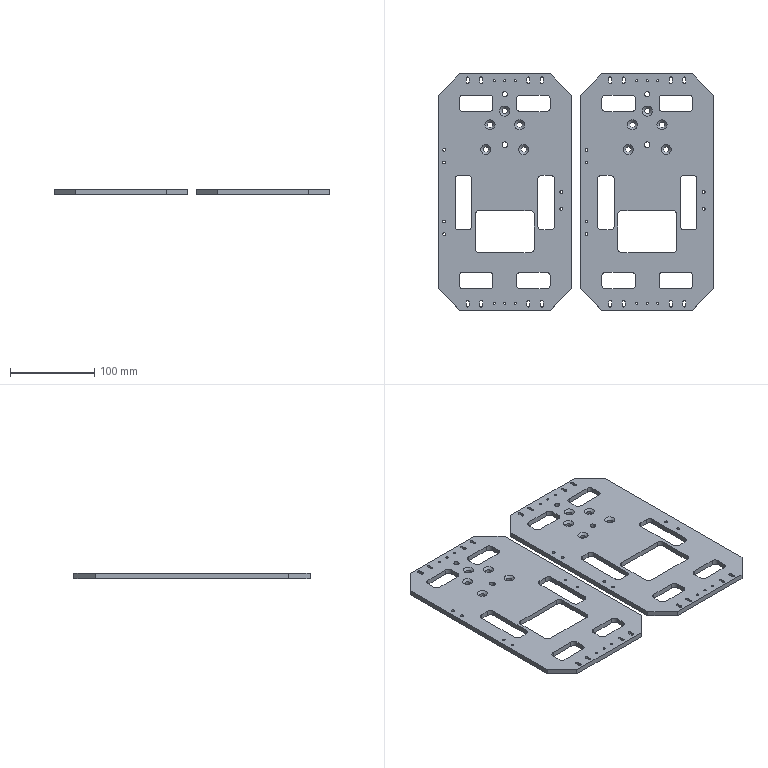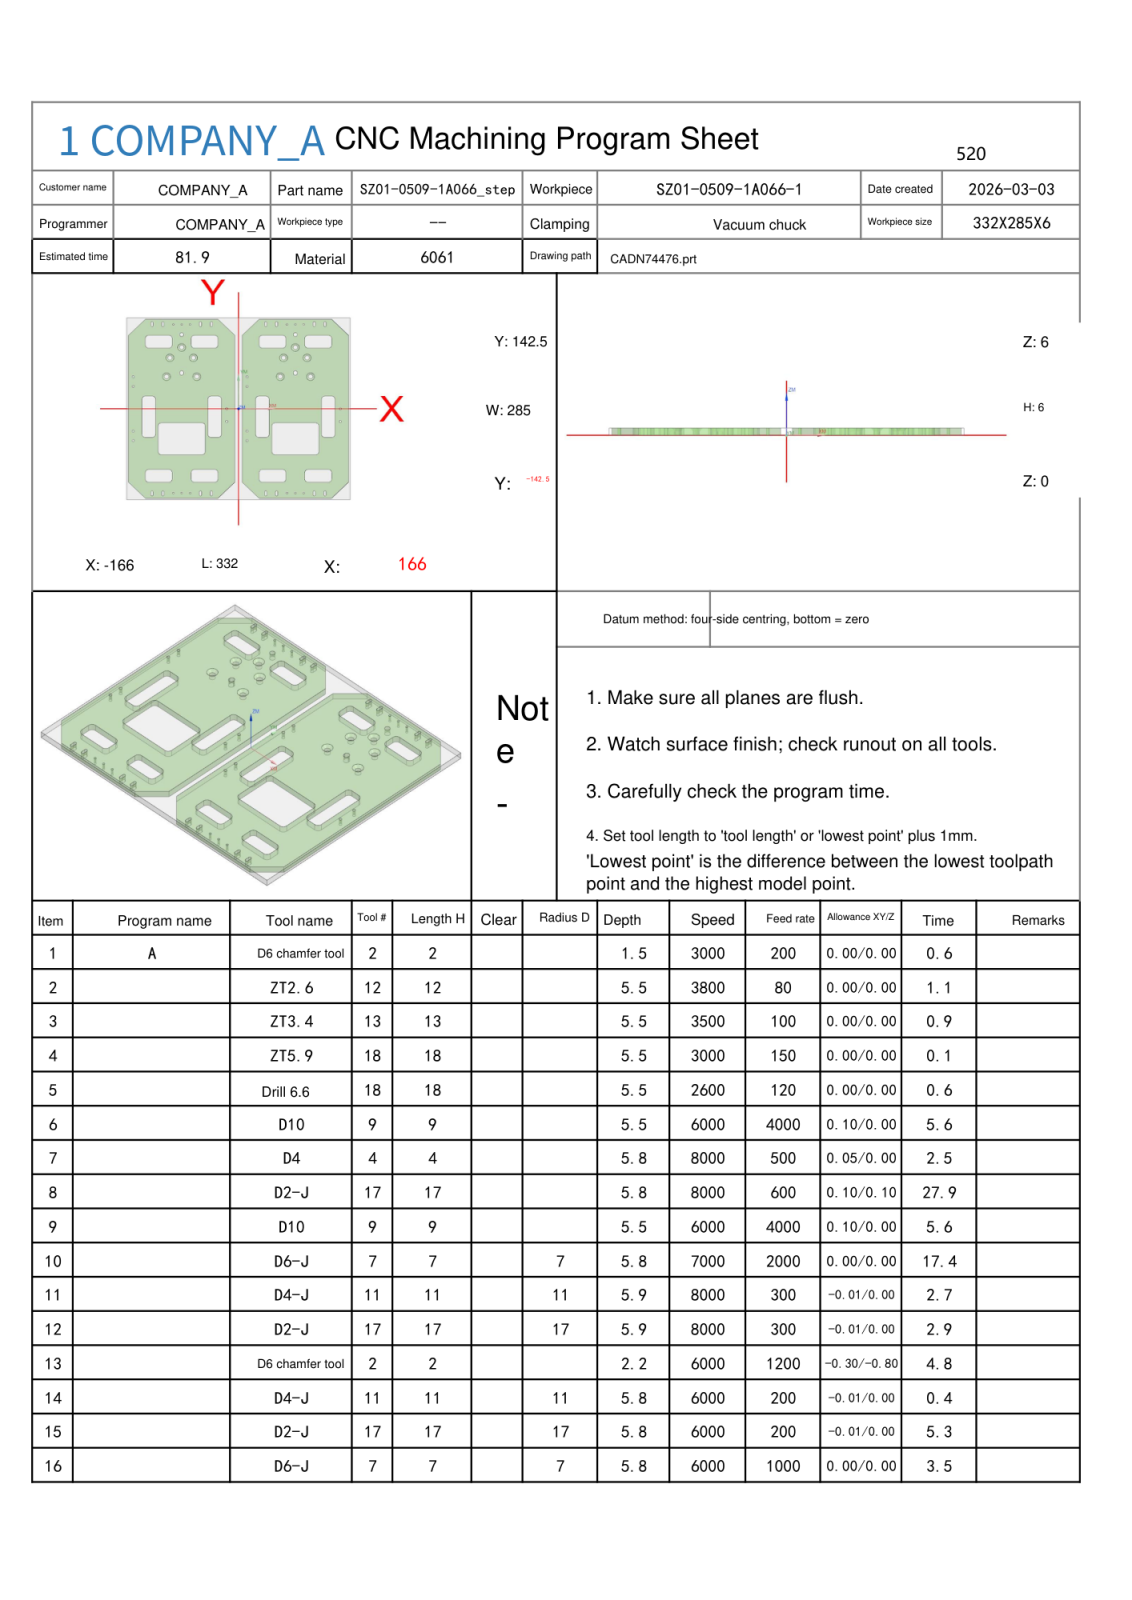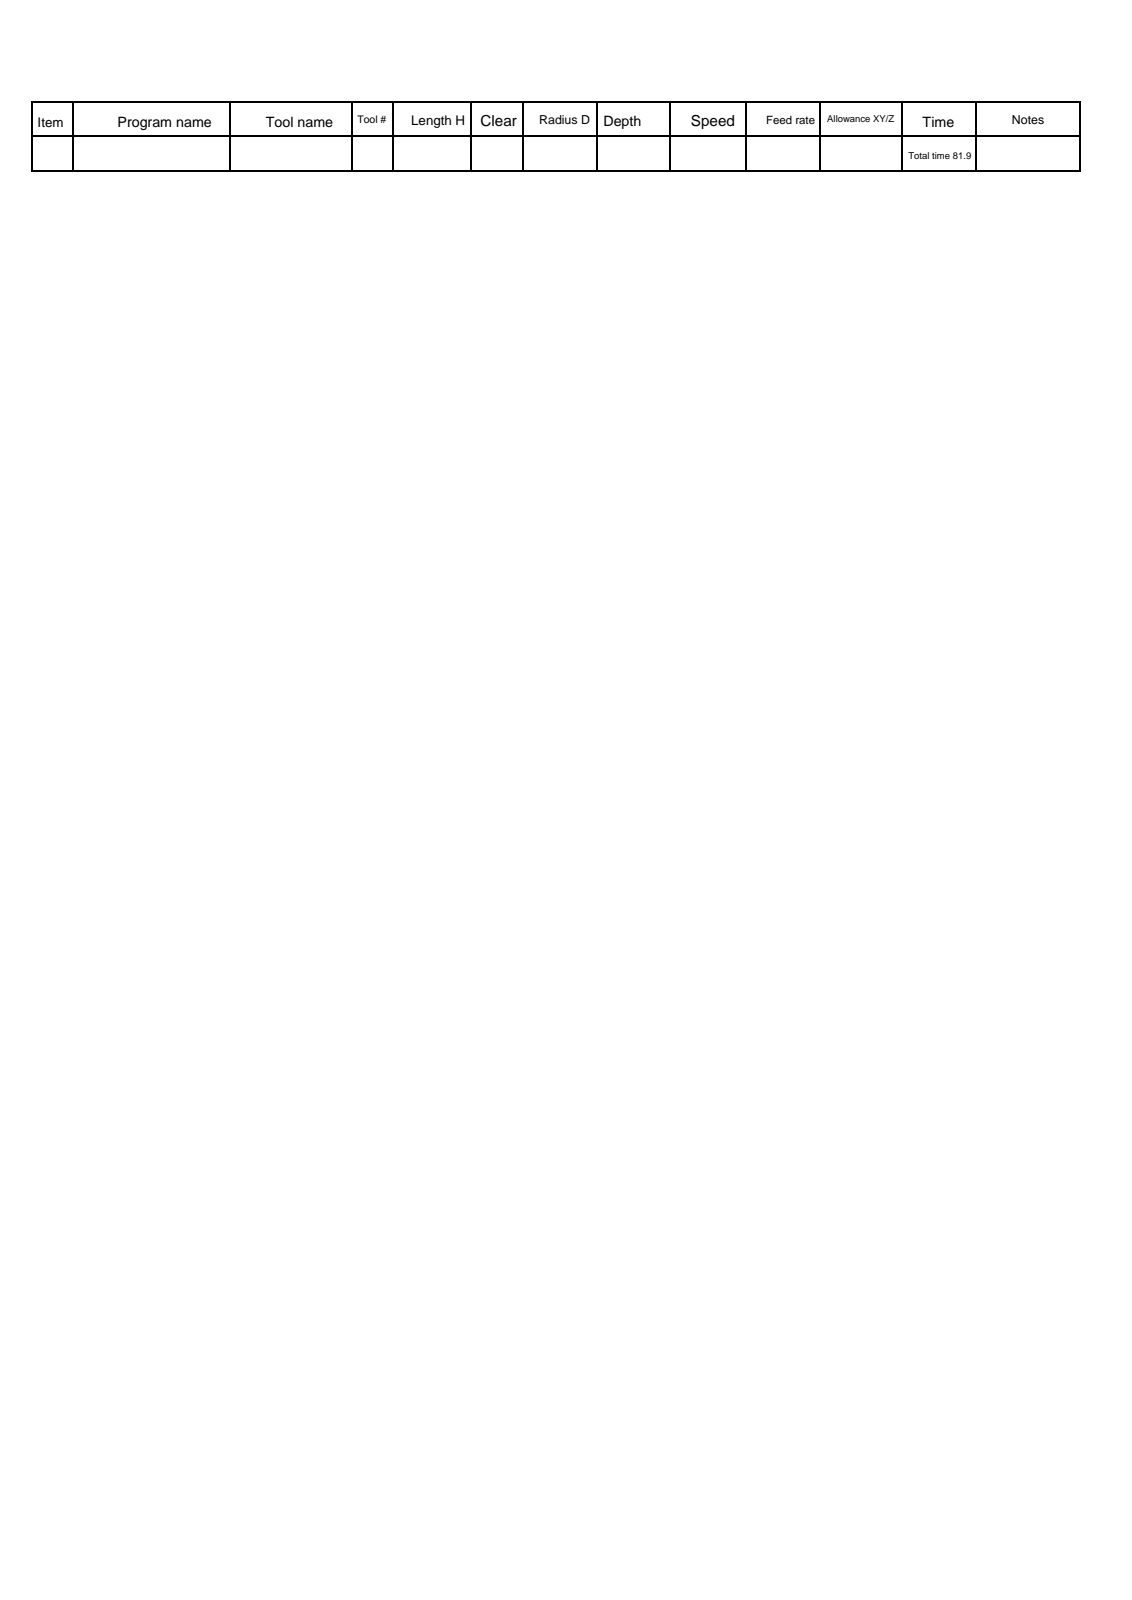NC program | NX | posted by the shop | part box 327 x 280 x 6 mm
Lines 1 to 1964 of 31860, first 1543 of 1962 lines:
%
O0001
(Machine time: 84.48 MIN)
(===Total Tool:9===)
(T2=D6 chamfer tool   D=6.   R=0.   D-  H02 Z=3.8   )
(T12=ZT2.6  D=2.6  DR_a=118 D-  H12 Z=0.5   )
(T13=ZT3.4  D=3.4  DR_a=118 D-  H13 Z=0.5   )
(T18=ZT5.9  D=5.9  DR_a=120 D-  H18 Z=0.5   )
(T9=D10     D=10.  R=0.   D-  H09 Z=0.5   )
(T4=D4      D=4.   R=0.   D-  H04 Z=0.2   )
(T17=D2-J   D=2.   R=0.   D-  H17 Z=0.15  )
(T7=D6-J    D=6.   R=0.   D7  H07 Z=0.2   )
(T11=D4-J   D=4.   R=0.   D11 H11 Z=0.15  )
G80 G90 G17 G49 G40
G91 G28 Z0
M01
N1 T02 M06
(D6 chamfer tool  D=6. R=0. H=02 ce=0.00 di=0.00)
G00 G90 G54 X97. Y132. M03 S3000
G43 H02 Z36.
M08
G98 G81 X97. Y132. Z5. R7. F200.
X84.5
X72.
X-72.
X-84.5
X-97.
Y-132.
X-84.5
X-72.
X72.
X84.5
X97.
G80
G00 Z36.
G00 G90 X-156.5 Y-50. M03 S3000
Z36.
G98 G81 X-156.5 Y-50. Z4.5 R7. F200.
Y-35.
Y35.
Y50.
X-107. Y50.25
X-102. Y79.75
X-84.5 Y116.
Y96.
X-67. Y79.75
X-62. Y50.25
X-17.5 Y0.0
Y-20.
X12.5 Y-50.
Y-35.
Y35.
Y50.
X62. Y50.25
X67. Y79.75
X84.5 Y96.
Y116.
X102. Y79.75
X107. Y50.25
X151.5 Y0.0
Y-20.
G80
G00 Z36.
G91 G28 Z0.0
M05
M09
G91 G28 Z0.0
M01
N2 T12 M06
(ZT2.6 D=2.6 DR_a=118 H=12)
G00 G90 G54 X97. Y132. M03 S3800
G43 H12 Z36.
M08
G98 G83 X97. Y132. Z.5 R7. F80. Q1.5
X84.5
X72.
X-72.
X-84.5
X-97.
Y-132.
X-84.5
X-72.
X72.
X84.5
X97.
G80
G00 Z36.
G91 G28 Z0.0
M05
M09
G91 G28 Z0.0
M01
N3 T13 M06
(ZT3.4 D=3.4 DR_a=118 H=13)
G00 G90 G54 X-17.5 Y-20. M03 S3500
G43 H13 Z36.
M08
G98 G83 X-17.5 Y-20. Z.5 R7. F100. Q1.5
Y0.0
X151.5
Y-20.
G80
G00 Z36.
G00 G90 X-156.5 Y50. M03 S3000
Z36.
G98 G83 X-156.5 Y50. Z.5 R7. F100. Q1.5
Y35.
Y-35.
Y-50.
X12.5
Y-35.
Y35.
Y50.
G80
G00 Z36.
G91 G28 Z0.0
M05
M09
G91 G28 Z0.0
M01
N4 T18 M06
(ZT5.9 D=5.9 DR_a=120 H=18)
G00 G90 G54 X-84.5 Y116. M03 S3000
G43 H18 Z36.
M08
G98 G83 X-84.5 Y116. Z.5 R7. F150. Q3.
X84.5
G80
G00 Z36.
G91 G28 Z0.0
M05
M09
G91 G28 Z0.0
M01
N5 T18 M06
(Drill 6.6 D=6.6 DR_a=120 H=18)
G00 G90 G54 X107. Y50.25 M03 S2600
G43 H18 Z36.
M08
G98 G83 X107. Y50.25 Z.5 R7. F120. Q1.5
X102. Y79.75
X84.5 Y96.
X67. Y79.75
X62. Y50.25
X-62.
X-67. Y79.75
X-84.5 Y96.
X-102. Y79.75
X-107. Y50.25
G80
G00 Z36.
G91 G28 Z0.0
M05
M09
G91 G28 Z0.0
M01
N6 T09 M06
(D10  D=10. R=0. H=09 ce=0.10 di=0.00)
G00 G90 G54 X84.5 Y-66.9 M03 S6000
G43 H09 Z36.
M08
Z6.5
G01 X114.4 Z6.431 F4000.
Y-27.1 Z6.339
X54.6 Z6.2
Y-66.9 Z6.108
X114.4 Z5.969
Y-27.1 Z5.877
X54.6 Z5.738
Y-66.9 Z5.646
X114.4 Z5.508
Y-27.1 Z5.415
X54.6 Z5.277
Y-66.9 Z5.185
X114.4 Z5.046
Y-27.1 Z4.954
X54.6 Z4.815
Y-66.9 Z4.723
X114.4 Z4.585
Y-27.1 Z4.492
X54.6 Z4.354
Y-66.9 Z4.262
X114.4 Z4.123
Y-27.1 Z4.031
X54.6 Z3.892
Y-66.9 Z3.8
X114.4 Z3.661
Y-27.1 Z3.569
X54.6 Z3.431
Y-66.9 Z3.339
X114.4 Z3.2
Y-27.1 Z3.108
X54.6 Z2.969
Y-66.9 Z2.877
X114.4 Z2.738
Y-27.1 Z2.646
X54.6 Z2.508
Y-66.9 Z2.415
X114.4 Z2.277
Y-27.1 Z2.185
X54.6 Z2.046
Y-66.9 Z1.954
X114.4 Z1.815
Y-27.1 Z1.723
X54.6 Z1.585
Y-66.9 Z1.492
X114.4 Z1.354
Y-27.1 Z1.262
X54.6 Z1.123
Y-66.9 Z1.031
X114.4 Z.892
Y-27.1 Z.8
X54.6 Z.661
Y-66.9 Z.569
X84.5 Z.5
X114.4
Y-27.1
X54.6
Y-66.9
X84.5
X85.
Z1.5
G00 Z36.
X-84.5
Z6.5
G01 X-54.6 Z6.431
Y-27.1 Z6.339
X-114.4 Z6.2
Y-66.9 Z6.108
X-54.6 Z5.969
Y-27.1 Z5.877
X-114.4 Z5.738
Y-66.9 Z5.646
X-54.6 Z5.508
Y-27.1 Z5.415
X-114.4 Z5.277
Y-66.9 Z5.185
X-54.6 Z5.046
Y-27.1 Z4.954
X-114.4 Z4.815
Y-66.9 Z4.723
X-54.6 Z4.585
Y-27.1 Z4.492
X-114.4 Z4.354
Y-66.9 Z4.262
X-54.6 Z4.123
Y-27.1 Z4.031
X-114.4 Z3.892
Y-66.9 Z3.8
X-54.6 Z3.661
Y-27.1 Z3.569
X-114.4 Z3.431
Y-66.9 Z3.339
X-54.6 Z3.2
Y-27.1 Z3.108
X-114.4 Z2.969
Y-66.9 Z2.877
X-54.6 Z2.738
Y-27.1 Z2.646
X-114.4 Z2.508
Y-66.9 Z2.415
X-54.6 Z2.277
Y-27.1 Z2.185
X-114.4 Z2.046
Y-66.9 Z1.954
X-54.6 Z1.815
Y-27.1 Z1.723
X-114.4 Z1.585
Y-66.9 Z1.492
X-54.6 Z1.354
Y-27.1 Z1.262
X-114.4 Z1.123
Y-66.9 Z1.031
X-54.6 Z.892
Y-27.1 Z.8
X-114.4 Z.661
Y-66.9 Z.569
X-84.5 Z.5
X-54.6
Y-27.1
X-114.4
Y-66.9
X-84.5
X-84.
Z1.5
G00 Z36.
G00 G90 X138.4 Y-12.5 M03 S6000
Z36.
Z6.5
G01 Y14.9 Z6.402 F4000.
X128.6 Z6.367
Y-39.9 Z6.171
X138.4 Z6.136
Y14.9 Z5.941
X128.6 Z5.906
Y-39.9 Z5.71
X138.4 Z5.675
Y14.9 Z5.479
X128.6 Z5.444
Y-39.9 Z5.248
X138.4 Z5.213
Y14.9 Z5.018
X128.6 Z4.982
Y-39.9 Z4.787
X138.4 Z4.752
Y14.9 Z4.556
X128.6 Z4.521
Y-39.9 Z4.325
X138.4 Z4.29
Y14.9 Z4.094
X128.6 Z4.059
Y-39.9 Z3.864
X138.4 Z3.829
Y14.9 Z3.633
X128.6 Z3.598
Y-39.9 Z3.402
X138.4 Z3.367
Y14.9 Z3.171
X128.6 Z3.136
Y-39.9 Z2.941
X138.4 Z2.906
Y14.9 Z2.71
X128.6 Z2.675
Y-39.9 Z2.479
X138.4 Z2.444
Y14.9 Z2.248
X128.6 Z2.213
Y-39.9 Z2.018
X138.4 Z1.982
Y14.9 Z1.787
X128.6 Z1.752
Y-39.9 Z1.556
X138.4 Z1.521
Y14.9 Z1.325
X128.6 Z1.29
Y-39.9 Z1.094
X138.4 Z1.059
Y14.9 Z.864
X128.6 Z.829
Y-39.9 Z.633
X138.4 Z.598
Y-12.5 Z.5
Y14.9
X128.6
Y-39.9
X138.4
Y-12.5
Y-12.
Z1.5
G00 Z36.
X40.4 Y-12.5
Z6.5
G01 Y14.9 Z6.402
X30.6 Z6.367
Y-39.9 Z6.171
X40.4 Z6.136
Y14.9 Z5.941
X30.6 Z5.906
Y-39.9 Z5.71
X40.4 Z5.675
Y14.9 Z5.479
X30.6 Z5.444
Y-39.9 Z5.248
X40.4 Z5.213
Y14.9 Z5.018
X30.6 Z4.982
Y-39.9 Z4.787
X40.4 Z4.752
Y14.9 Z4.556
X30.6 Z4.521
Y-39.9 Z4.325
X40.4 Z4.29
Y14.9 Z4.094
X30.6 Z4.059
Y-39.9 Z3.864
X40.4 Z3.829
Y14.9 Z3.633
X30.6 Z3.598
Y-39.9 Z3.402
X40.4 Z3.367
Y14.9 Z3.171
X30.6 Z3.136
Y-39.9 Z2.941
X40.4 Z2.906
Y14.9 Z2.71
X30.6 Z2.675
Y-39.9 Z2.479
X40.4 Z2.444
Y14.9 Z2.248
X30.6 Z2.213
Y-39.9 Z2.018
X40.4 Z1.982
Y14.9 Z1.787
X30.6 Z1.752
Y-39.9 Z1.556
X40.4 Z1.521
Y14.9 Z1.325
X30.6 Z1.29
Y-39.9 Z1.094
X40.4 Z1.059
Y14.9 Z.864
X30.6 Z.829
Y-39.9 Z.633
X40.4 Z.598
Y-12.5 Z.5
Y14.9
X30.6
Y-39.9
X40.4
Y-12.5
Y-12.
Z1.5
G00 Z36.
X-30.6 Y-12.5
Z6.5
G01 Y14.9 Z6.402
X-40.4 Z6.367
Y-39.9 Z6.171
X-30.6 Z6.136
Y14.9 Z5.941
X-40.4 Z5.906
Y-39.9 Z5.71
X-30.6 Z5.675
Y14.9 Z5.479
X-40.4 Z5.444
Y-39.9 Z5.248
X-30.6 Z5.213
Y14.9 Z5.018
X-40.4 Z4.982
Y-39.9 Z4.787
X-30.6 Z4.752
Y14.9 Z4.556
X-40.4 Z4.521
Y-39.9 Z4.325
X-30.6 Z4.29
Y14.9 Z4.094
X-40.4 Z4.059
Y-39.9 Z3.864
X-30.6 Z3.829
Y14.9 Z3.633
X-40.4 Z3.598
Y-39.9 Z3.402
X-30.6 Z3.367
Y14.9 Z3.171
X-40.4 Z3.136
Y-39.9 Z2.941
X-30.6 Z2.906
Y14.9 Z2.71
X-40.4 Z2.675
Y-39.9 Z2.479
X-30.6 Z2.444
Y14.9 Z2.248
X-40.4 Z2.213
Y-39.9 Z2.018
X-30.6 Z1.982
Y14.9 Z1.787
X-40.4 Z1.752
Y-39.9 Z1.556
X-30.6 Z1.521
Y14.9 Z1.325
X-40.4 Z1.29
Y-39.9 Z1.094
X-30.6 Z1.059
Y14.9 Z.864
X-40.4 Z.829
Y-39.9 Z.633
X-30.6 Z.598
Y-12.5 Z.5
Y14.9
X-40.4
Y-39.9
X-30.6
Y-12.5
Y-12.
Z1.5
G00 Z36.
X-138.4 Y-12.5
Z6.5
G01 Y-39.9 Z6.402
X-128.6 Z6.367
Y14.9 Z6.171
X-138.4 Z6.136
Y-39.9 Z5.941
X-128.6 Z5.906
Y14.9 Z5.71
X-138.4 Z5.675
Y-39.9 Z5.479
X-128.6 Z5.444
Y14.9 Z5.248
X-138.4 Z5.213
Y-39.9 Z5.018
X-128.6 Z4.982
Y14.9 Z4.787
X-138.4 Z4.752
Y-39.9 Z4.556
X-128.6 Z4.521
Y14.9 Z4.325
X-138.4 Z4.29
Y-39.9 Z4.094
X-128.6 Z4.059
Y14.9 Z3.864
X-138.4 Z3.829
Y-39.9 Z3.633
X-128.6 Z3.598
Y14.9 Z3.402
X-138.4 Z3.367
Y-39.9 Z3.171
X-128.6 Z3.136
Y14.9 Z2.941
X-138.4 Z2.906
Y-39.9 Z2.71
X-128.6 Z2.675
Y14.9 Z2.479
X-138.4 Z2.444
Y-39.9 Z2.248
X-128.6 Z2.213
Y14.9 Z2.018
X-138.4 Z1.982
Y-39.9 Z1.787
X-128.6 Z1.752
Y14.9 Z1.556
X-138.4 Z1.521
Y-39.9 Z1.325
X-128.6 Z1.29
Y14.9 Z1.094
X-138.4 Z1.059
Y-39.9 Z.864
X-128.6 Z.829
Y14.9 Z.633
X-138.4 Z.598
Y-12.5 Z.5
Y-39.9
X-128.6
Y14.9
X-138.4
Y-12.5
Y-13.
Z1.5
G00 Z36.
G00 G90 X-118.5 Y109.9 M03 S6000
Z36.
Z6.5
G01 X-133.4 Z6.413 F4000.
Y100.1 Z6.356
X-103.6 Z6.182
Y109.9 Z6.125
X-133.4 Z5.952
Y100.1 Z5.895
X-103.6 Z5.721
Y109.9 Z5.664
X-133.4 Z5.49
Y100.1 Z5.433
X-103.6 Z5.259
Y109.9 Z5.202
X-133.4 Z5.029
Y100.1 Z4.971
X-103.6 Z4.798
Y109.9 Z4.741
X-133.4 Z4.567
Y100.1 Z4.51
X-103.6 Z4.336
Y109.9 Z4.279
X-133.4 Z4.105
Y100.1 Z4.048
X-103.6 Z3.875
Y109.9 Z3.818
X-133.4 Z3.644
Y100.1 Z3.587
X-103.6 Z3.413
Y109.9 Z3.356
X-133.4 Z3.182
Y100.1 Z3.125
X-103.6 Z2.952
Y109.9 Z2.895
X-133.4 Z2.721
Y100.1 Z2.664
X-103.6 Z2.49
Y109.9 Z2.433
X-133.4 Z2.259
Y100.1 Z2.202
X-103.6 Z2.029
Y109.9 Z1.971
X-133.4 Z1.798
Y100.1 Z1.741
X-103.6 Z1.567
Y109.9 Z1.51
X-133.4 Z1.336
Y100.1 Z1.279
X-103.6 Z1.105
Y109.9 Z1.048
X-133.4 Z.875
Y100.1 Z.818
X-103.6 Z.644
Y109.9 Z.587
X-118.5 Z.5
X-133.4
Y100.1
X-103.6
Y109.9
X-118.5
X-119.
Z1.5
G00 Z36.
X-50.5
Z6.5
G01 X-65.4 Z6.413
Y100.1 Z6.356
X-35.6 Z6.182
Y109.9 Z6.125
X-65.4 Z5.952
Y100.1 Z5.895
X-35.6 Z5.721
Y109.9 Z5.664
X-65.4 Z5.49
Y100.1 Z5.433
X-35.6 Z5.259
Y109.9 Z5.202
X-65.4 Z5.029
Y100.1 Z4.971
X-35.6 Z4.798
Y109.9 Z4.741
X-65.4 Z4.567
Y100.1 Z4.51
X-35.6 Z4.336
Y109.9 Z4.279
X-65.4 Z4.105
Y100.1 Z4.048
X-35.6 Z3.875
Y109.9 Z3.818
X-65.4 Z3.644
Y100.1 Z3.587
X-35.6 Z3.413
Y109.9 Z3.356
X-65.4 Z3.182
Y100.1 Z3.125
X-35.6 Z2.952
Y109.9 Z2.895
X-65.4 Z2.721
Y100.1 Z2.664
X-35.6 Z2.49
Y109.9 Z2.433
X-65.4 Z2.259
Y100.1 Z2.202
X-35.6 Z2.029
Y109.9 Z1.971
X-65.4 Z1.798
Y100.1 Z1.741
X-35.6 Z1.567
Y109.9 Z1.51
X-65.4 Z1.336
Y100.1 Z1.279
X-35.6 Z1.105
Y109.9 Z1.048
X-65.4 Z.875
Y100.1 Z.818
X-35.6 Z.644
Y109.9 Z.587
X-50.5 Z.5
X-65.4
Y100.1
X-35.6
Y109.9
X-50.5
X-51.
Z1.5
G00 Z36.
X50.5
Z6.5
G01 X35.6 Z6.413
Y100.1 Z6.356
X65.4 Z6.182
Y109.9 Z6.125
X35.6 Z5.952
Y100.1 Z5.895
X65.4 Z5.721
Y109.9 Z5.664
X35.6 Z5.49
Y100.1 Z5.433
X65.4 Z5.259
Y109.9 Z5.202
X35.6 Z5.029
Y100.1 Z4.971
X65.4 Z4.798
Y109.9 Z4.741
X35.6 Z4.567
Y100.1 Z4.51
X65.4 Z4.336
Y109.9 Z4.279
X35.6 Z4.105
Y100.1 Z4.048
X65.4 Z3.875
Y109.9 Z3.818
X35.6 Z3.644
Y100.1 Z3.587
X65.4 Z3.413
Y109.9 Z3.356
X35.6 Z3.182
Y100.1 Z3.125
X65.4 Z2.952
Y109.9 Z2.895
X35.6 Z2.721
Y100.1 Z2.664
X65.4 Z2.49
Y109.9 Z2.433
X35.6 Z2.259
Y100.1 Z2.202
X65.4 Z2.029
Y109.9 Z1.971
X35.6 Z1.798
Y100.1 Z1.741
X65.4 Z1.567
Y109.9 Z1.51
X35.6 Z1.336
Y100.1 Z1.279
X65.4 Z1.105
Y109.9 Z1.048
X35.6 Z.875
Y100.1 Z.818
X65.4 Z.644
Y109.9 Z.587
X50.5 Z.5
X35.6
Y100.1
X65.4
Y109.9
X50.5
X50.
Z1.5
G00 Z36.
X118.5
Z6.5
G01 X103.6 Z6.413
Y100.1 Z6.356
X133.4 Z6.182
Y109.9 Z6.125
X103.6 Z5.952
Y100.1 Z5.895
X133.4 Z5.721
Y109.9 Z5.664
X103.6 Z5.49
Y100.1 Z5.433
X133.4 Z5.259
Y109.9 Z5.202
X103.6 Z5.029
Y100.1 Z4.971
X133.4 Z4.798
Y109.9 Z4.741
X103.6 Z4.567
Y100.1 Z4.51
X133.4 Z4.336
Y109.9 Z4.279
X103.6 Z4.105
Y100.1 Z4.048
X133.4 Z3.875
Y109.9 Z3.818
X103.6 Z3.644
Y100.1 Z3.587
X133.4 Z3.413
Y109.9 Z3.356
X103.6 Z3.182
Y100.1 Z3.125
X133.4 Z2.952
Y109.9 Z2.895
X103.6 Z2.721
Y100.1 Z2.664
X133.4 Z2.49
Y109.9 Z2.433
X103.6 Z2.259
Y100.1 Z2.202
X133.4 Z2.029
Y109.9 Z1.971
X103.6 Z1.798
Y100.1 Z1.741
X133.4 Z1.567
Y109.9 Z1.51
X103.6 Z1.336
Y100.1 Z1.279
X133.4 Z1.105
Y109.9 Z1.048
X103.6 Z.875
Y100.1 Z.818
X133.4 Z.644
Y109.9 Z.587
X118.5 Z.5
X103.6
Y100.1
X133.4
Y109.9
X118.5
X118.
Z1.5
G00 Z36.
X118.5 Y-109.9
Z6.5
G01 X133.4 Z6.413
Y-100.1 Z6.356
X103.6 Z6.182
Y-109.9 Z6.125
X133.4 Z5.952
Y-100.1 Z5.895
X103.6 Z5.721
Y-109.9 Z5.664
X133.4 Z5.49
Y-100.1 Z5.433
X103.6 Z5.259
Y-109.9 Z5.202
X133.4 Z5.029
Y-100.1 Z4.971
X103.6 Z4.798
Y-109.9 Z4.741
X133.4 Z4.567
Y-100.1 Z4.51
X103.6 Z4.336
Y-109.9 Z4.279
X133.4 Z4.105
Y-100.1 Z4.048
X103.6 Z3.875
Y-109.9 Z3.818
X133.4 Z3.644
Y-100.1 Z3.587
X103.6 Z3.413
Y-109.9 Z3.356
X133.4 Z3.182
Y-100.1 Z3.125
X103.6 Z2.952
Y-109.9 Z2.895
X133.4 Z2.721
Y-100.1 Z2.664
X103.6 Z2.49
Y-109.9 Z2.433
X133.4 Z2.259
Y-100.1 Z2.202
X103.6 Z2.029
Y-109.9 Z1.971
X133.4 Z1.798
Y-100.1 Z1.741
X103.6 Z1.567
Y-109.9 Z1.51
X133.4 Z1.336
Y-100.1 Z1.279
X103.6 Z1.105
Y-109.9 Z1.048
X133.4 Z.875
Y-100.1 Z.818
X103.6 Z.644
Y-109.9 Z.587
X118.5 Z.5
X133.4
Y-100.1
X103.6
Y-109.9
X118.5
X119.
Z1.5
G00 Z36.
X50.5
Z6.5
G01 X65.4 Z6.413
Y-100.1 Z6.356
X35.6 Z6.182
Y-109.9 Z6.125
X65.4 Z5.952
Y-100.1 Z5.895
X35.6 Z5.721
Y-109.9 Z5.664
X65.4 Z5.49
Y-100.1 Z5.433
X35.6 Z5.259
Y-109.9 Z5.202
X65.4 Z5.029
Y-100.1 Z4.971
X35.6 Z4.798
Y-109.9 Z4.741
X65.4 Z4.567
Y-100.1 Z4.51
X35.6 Z4.336
Y-109.9 Z4.279
X65.4 Z4.105
Y-100.1 Z4.048
X35.6 Z3.875
Y-109.9 Z3.818
X65.4 Z3.644
Y-100.1 Z3.587
X35.6 Z3.413
Y-109.9 Z3.356
X65.4 Z3.182
Y-100.1 Z3.125
X35.6 Z2.952
Y-109.9 Z2.895
X65.4 Z2.721
Y-100.1 Z2.664
X35.6 Z2.49
Y-109.9 Z2.433
X65.4 Z2.259
Y-100.1 Z2.202
X35.6 Z2.029
Y-109.9 Z1.971
X65.4 Z1.798
Y-100.1 Z1.741
X35.6 Z1.567
Y-109.9 Z1.51
X65.4 Z1.336
Y-100.1 Z1.279
X35.6 Z1.105
Y-109.9 Z1.048
X65.4 Z.875
Y-100.1 Z.818
X35.6 Z.644
Y-109.9 Z.587
X50.5 Z.5
X65.4
Y-100.1
X35.6
Y-109.9
X50.5
X51.
Z1.5
G00 Z36.
X-50.5
Z6.5
G01 X-35.6 Z6.413
Y-100.1 Z6.356
X-65.4 Z6.182
Y-109.9 Z6.125
X-35.6 Z5.952
Y-100.1 Z5.895
X-65.4 Z5.721
Y-109.9 Z5.664
X-35.6 Z5.49
Y-100.1 Z5.433
X-65.4 Z5.259
Y-109.9 Z5.202
X-35.6 Z5.029
Y-100.1 Z4.971
X-65.4 Z4.798
Y-109.9 Z4.741
X-35.6 Z4.567
Y-100.1 Z4.51
X-65.4 Z4.336
Y-109.9 Z4.279
X-35.6 Z4.105
Y-100.1 Z4.048
X-65.4 Z3.875
Y-109.9 Z3.818
X-35.6 Z3.644
Y-100.1 Z3.587
X-65.4 Z3.413
Y-109.9 Z3.356
X-35.6 Z3.182
Y-100.1 Z3.125
X-65.4 Z2.952
Y-109.9 Z2.895
X-35.6 Z2.721
Y-100.1 Z2.664
X-65.4 Z2.49
Y-109.9 Z2.433
X-35.6 Z2.259
Y-100.1 Z2.202
X-65.4 Z2.029
Y-109.9 Z1.971
X-35.6 Z1.798
Y-100.1 Z1.741
X-65.4 Z1.567
Y-109.9 Z1.51
X-35.6 Z1.336
Y-100.1 Z1.279
X-65.4 Z1.105
Y-109.9 Z1.048
X-35.6 Z.875
Y-100.1 Z.818
X-65.4 Z.644
Y-109.9 Z.587
X-50.5 Z.5
X-35.6
Y-100.1
X-65.4
Y-109.9
X-50.5
X-50.
Z1.5
G00 Z36.
X-118.5
Z6.5
G01 X-103.6 Z6.413
Y-100.1 Z6.356
X-133.4 Z6.182
Y-109.9 Z6.125
X-103.6 Z5.952
Y-100.1 Z5.895
X-133.4 Z5.721
Y-109.9 Z5.664
X-103.6 Z5.49
Y-100.1 Z5.433
X-133.4 Z5.259
Y-109.9 Z5.202
X-103.6 Z5.029
Y-100.1 Z4.971
X-133.4 Z4.798
Y-109.9 Z4.741
X-103.6 Z4.567
Y-100.1 Z4.51
X-133.4 Z4.336
Y-109.9 Z4.279
X-103.6 Z4.105
Y-100.1 Z4.048
X-133.4 Z3.875
Y-109.9 Z3.818
X-103.6 Z3.644
Y-100.1 Z3.587
X-133.4 Z3.413
Y-109.9 Z3.356
X-103.6 Z3.182
Y-100.1 Z3.125
X-133.4 Z2.952
Y-109.9 Z2.895
X-103.6 Z2.721
Y-100.1 Z2.664
X-133.4 Z2.49
Y-109.9 Z2.433
X-103.6 Z2.259
Y-100.1 Z2.202
X-133.4 Z2.029
Y-109.9 Z1.971
X-103.6 Z1.798
Y-100.1 Z1.741
X-133.4 Z1.567
Y-109.9 Z1.51
X-103.6 Z1.336
Y-100.1 Z1.279
X-133.4 Z1.105
Y-109.9 Z1.048
X-103.6 Z.875
Y-100.1 Z.818
X-133.4 Z.644
Y-109.9 Z.587
X-118.5 Z.5
X-103.6
Y-100.1
X-133.4
Y-109.9
X-118.5
X-118.
Z1.5
G00 Z36.
G91 G28 Z0.0
M05
M09
G91 G28 Z0.0
M01
N7 T04 M06
(D4  D=4. R=0. H=04 ce=0.05 di=0.00)
G00 G90 G54 X-84.5 Y116.95 M03 S8000
G43 H04 Z36.
M08
Z6.5
G03 X-85.45 Y116. Z6.463 I0.0 J-.95 F500.
X-84.5 Y115.05 Z6.427 I.95 J0.0
X-83.55 Y116. Z6.39 I0.0 J.95
X-84.5 Y116.95 Z6.353 I-.95 J0.0
X-85.45 Y116. Z6.317 I0.0 J-.95
X-84.5 Y115.05 Z6.28 I.95 J0.0
X-83.55 Y116. Z6.244 I0.0 J.95
X-84.5 Y116.95 Z6.207 I-.95 J0.0
X-85.45 Y116. Z6.17 I0.0 J-.95
X-84.5 Y115.05 Z6.134 I.95 J0.0
X-83.55 Y116. Z6.097 I0.0 J.95
X-84.5 Y116.95 Z6.06 I-.95 J0.0
X-85.45 Y116. Z6.024 I0.0 J-.95
X-84.5 Y115.05 Z5.987 I.95 J0.0
X-83.55 Y116. Z5.951 I0.0 J.95
X-84.5 Y116.95 Z5.914 I-.95 J0.0
X-85.45 Y116. Z5.877 I0.0 J-.95
X-84.5 Y115.05 Z5.841 I.95 J0.0
X-83.55 Y116. Z5.804 I0.0 J.95
X-84.5 Y116.95 Z5.767 I-.95 J0.0
X-85.45 Y116. Z5.731 I0.0 J-.95
X-84.5 Y115.05 Z5.694 I.95 J0.0
X-83.55 Y116. Z5.658 I0.0 J.95
X-84.5 Y116.95 Z5.621 I-.95 J0.0
X-85.45 Y116. Z5.584 I0.0 J-.95
X-84.5 Y115.05 Z5.548 I.95 J0.0
X-83.55 Y116. Z5.511 I0.0 J.95
X-84.5 Y116.95 Z5.474 I-.95 J0.0
X-85.45 Y116. Z5.438 I0.0 J-.95
X-84.5 Y115.05 Z5.401 I.95 J0.0
X-83.55 Y116. Z5.365 I0.0 J.95
X-84.5 Y116.95 Z5.328 I-.95 J0.0
X-85.45 Y116. Z5.291 I0.0 J-.95
X-84.5 Y115.05 Z5.255 I.95 J0.0
X-83.55 Y116. Z5.218 I0.0 J.95
X-84.5 Y116.95 Z5.181 I-.95 J0.0
X-85.45 Y116. Z5.145 I0.0 J-.95
X-84.5 Y115.05 Z5.108 I.95 J0.0
X-83.55 Y116. Z5.072 I0.0 J.95
X-84.5 Y116.95 Z5.035 I-.95 J0.0
X-85.45 Y116. Z4.998 I0.0 J-.95
X-84.5 Y115.05 Z4.962 I.95 J0.0
X-83.55 Y116. Z4.925 I0.0 J.95
X-84.5 Y116.95 Z4.888 I-.95 J0.0
X-85.45 Y116. Z4.852 I0.0 J-.95
X-84.5 Y115.05 Z4.815 I.95 J0.0
X-83.55 Y116. Z4.778 I0.0 J.95
X-84.5 Y116.95 Z4.742 I-.95 J0.0
X-85.45 Y116. Z4.705 I0.0 J-.95
X-84.5 Y115.05 Z4.669 I.95 J0.0
X-83.55 Y116. Z4.632 I0.0 J.95
X-84.5 Y116.95 Z4.595 I-.95 J0.0
X-85.45 Y116. Z4.559 I0.0 J-.95
X-84.5 Y115.05 Z4.522 I.95 J0.0
X-83.55 Y116. Z4.485 I0.0 J.95
X-84.5 Y116.95 Z4.449 I-.95 J0.0
X-85.45 Y116. Z4.412 I0.0 J-.95
X-84.5 Y115.05 Z4.376 I.95 J0.0
X-83.55 Y116. Z4.339 I0.0 J.95
X-84.5 Y116.95 Z4.302 I-.95 J0.0
X-85.45 Y116. Z4.266 I0.0 J-.95
X-84.5 Y115.05 Z4.229 I.95 J0.0
X-83.55 Y116. Z4.192 I0.0 J.95
X-84.5 Y116.95 Z4.156 I-.95 J0.0
X-85.45 Y116. Z4.119 I0.0 J-.95
X-84.5 Y115.05 Z4.083 I.95 J0.0
X-83.55 Y116. Z4.046 I0.0 J.95
X-84.5 Y116.95 Z4.009 I-.95 J0.0
X-85.45 Y116. Z3.973 I0.0 J-.95
X-84.5 Y115.05 Z3.936 I.95 J0.0
X-83.55 Y116. Z3.899 I0.0 J.95
X-84.5 Y116.95 Z3.863 I-.95 J0.0
X-85.45 Y116. Z3.826 I0.0 J-.95
X-84.5 Y115.05 Z3.79 I.95 J0.0
X-83.55 Y116. Z3.753 I0.0 J.95
X-84.5 Y116.95 Z3.716 I-.95 J0.0
X-85.45 Y116. Z3.68 I0.0 J-.95
X-84.5 Y115.05 Z3.643 I.95 J0.0
X-83.55 Y116. Z3.606 I0.0 J.95
X-84.5 Y116.95 Z3.57 I-.95 J0.0
X-85.45 Y116. Z3.533 I0.0 J-.95
X-84.5 Y115.05 Z3.497 I.95 J0.0
X-83.55 Y116. Z3.46 I0.0 J.95
X-84.5 Y116.95 Z3.423 I-.95 J0.0
X-85.45 Y116. Z3.387 I0.0 J-.95
X-84.5 Y115.05 Z3.35 I.95 J0.0
X-83.55 Y116. Z3.313 I0.0 J.95
X-84.5 Y116.95 Z3.277 I-.95 J0.0
X-85.45 Y116. Z3.24 I0.0 J-.95
X-84.5 Y115.05 Z3.203 I.95 J0.0
X-83.55 Y116. Z3.167 I0.0 J.95
X-84.5 Y116.95 Z3.13 I-.95 J0.0
X-85.45 Y116. Z3.094 I0.0 J-.95
X-84.5 Y115.05 Z3.057 I.95 J0.0
X-83.55 Y116. Z3.02 I0.0 J.95
X-84.5 Y116.95 Z2.984 I-.95 J0.0
X-85.45 Y116. Z2.947 I0.0 J-.95
X-84.5 Y115.05 Z2.91 I.95 J0.0
X-83.55 Y116. Z2.874 I0.0 J.95
X-84.5 Y116.95 Z2.837 I-.95 J0.0
X-85.45 Y116. Z2.801 I0.0 J-.95
X-84.5 Y115.05 Z2.764 I.95 J0.0
X-83.55 Y116. Z2.727 I0.0 J.95
X-84.5 Y116.95 Z2.691 I-.95 J0.0
X-85.45 Y116. Z2.654 I0.0 J-.95
X-84.5 Y115.05 Z2.617 I.95 J0.0
X-83.55 Y116. Z2.581 I0.0 J.95
X-84.5 Y116.95 Z2.544 I-.95 J0.0
X-85.45 Y116. Z2.508 I0.0 J-.95
X-84.5 Y115.05 Z2.471 I.95 J0.0
X-83.55 Y116. Z2.434 I0.0 J.95
X-84.5 Y116.95 Z2.398 I-.95 J0.0
X-85.45 Y116. Z2.361 I0.0 J-.95
X-84.5 Y115.05 Z2.324 I.95 J0.0
X-83.55 Y116. Z2.288 I0.0 J.95
X-84.5 Y116.95 Z2.251 I-.95 J0.0
X-85.45 Y116. Z2.215 I0.0 J-.95
X-84.5 Y115.05 Z2.178 I.95 J0.0
X-83.55 Y116. Z2.141 I0.0 J.95
X-84.5 Y116.95 Z2.105 I-.95 J0.0
X-85.45 Y116. Z2.068 I0.0 J-.95
X-84.5 Y115.05 Z2.031 I.95 J0.0
X-83.55 Y116. Z1.995 I0.0 J.95
X-84.5 Y116.95 Z1.958 I-.95 J0.0
X-85.45 Y116. Z1.922 I0.0 J-.95
X-84.5 Y115.05 Z1.885 I.95 J0.0
X-83.55 Y116. Z1.848 I0.0 J.95
X-84.5 Y116.95 Z1.812 I-.95 J0.0
X-85.45 Y116. Z1.775 I0.0 J-.95
X-84.5 Y115.05 Z1.738 I.95 J0.0
X-83.55 Y116. Z1.702 I0.0 J.95
X-84.5 Y116.95 Z1.665 I-.95 J0.0
X-85.45 Y116. Z1.628 I0.0 J-.95
X-84.5 Y115.05 Z1.592 I.95 J0.0
X-83.55 Y116. Z1.555 I0.0 J.95
X-84.5 Y116.95 Z1.519 I-.95 J0.0
X-85.45 Y116. Z1.482 I0.0 J-.95
X-84.5 Y115.05 Z1.445 I.95 J0.0
X-83.55 Y116. Z1.409 I0.0 J.95
X-84.5 Y116.95 Z1.372 I-.95 J0.0
X-85.45 Y116. Z1.335 I0.0 J-.95
X-84.5 Y115.05 Z1.299 I.95 J0.0
X-83.55 Y116. Z1.262 I0.0 J.95
X-84.5 Y116.95 Z1.226 I-.95 J0.0
X-85.45 Y116. Z1.189 I0.0 J-.95
X-84.5 Y115.05 Z1.152 I.95 J0.0
X-83.55 Y116. Z1.116 I0.0 J.95
X-84.5 Y116.95 Z1.079 I-.95 J0.0
X-85.45 Y116. Z1.042 I0.0 J-.95
X-84.5 Y115.05 Z1.006 I.95 J0.0
X-83.55 Y116. Z.969 I0.0 J.95
X-84.5 Y116.95 Z.933 I-.95 J0.0
X-85.45 Y116. Z.896 I0.0 J-.95
X-84.5 Y115.05 Z.859 I.95 J0.0
X-83.55 Y116. Z.823 I0.0 J.95
X-84.5 Y116.95 Z.786 I-.95 J0.0
X-85.45 Y116. Z.749 I0.0 J-.95
X-84.5 Y115.05 Z.713 I.95 J0.0
X-83.55 Y116. Z.676 I0.0 J.95
X-84.5 Y116.95 Z.64 I-.95 J0.0
X-85.45 Y116. Z.603 I0.0 J-.95
X-84.5 Y115.05 Z.566 I.95 J0.0
X-83.55 Y116. Z.53 I0.0 J.95
X-84.5 Y116.95 Z.493 I-.95 J0.0
X-85.45 Y116. Z.456 I0.0 J-.95
X-84.5 Y115.05 Z.42 I.95 J0.0
X-83.55 Y116. Z.383 I0.0 J.95
X-84.5 Y116.95 Z.347 I-.95 J0.0
X-85.45 Y116. Z.31 I0.0 J-.95
X-84.5 Y115.05 Z.273 I.95 J0.0
X-83.55 Y116. Z.237 I0.0 J.95
X-84.5 Y116.95 Z.2 I-.95 J0.0
X-85.45 Y116. I0.0 J-.95
X-84.5 Y115.05 I.95 J0.0
X-83.55 Y116. I0.0 J.95
X-84.5 Y116.95 I-.95 J0.0
X-84.977 Y116.821 I0.0 J-.95
G01 Z1.2
G00 Z36.
X-85.45 Y56.
Z6.5
G01 Y55.5 Z6.491
G03 X-84.5 Y54.55 Z6.463 I.95 J0.0
X-83.55 Y55.5 Z6.436 I0.0 J.95
G01 Y56.5 Z6.418
G03 X-84.5 Y57.45 Z6.39 I-.95 J0.0
X-85.45 Y56.5 Z6.363 I0.0 J-.95
G01 Y55.5 Z6.344
G03 X-84.5 Y54.55 Z6.317 I.95 J0.0
X-83.55 Y55.5 Z6.289 I0.0 J.95
G01 Y56.5 Z6.271
G03 X-84.5 Y57.45 Z6.244 I-.95 J0.0
X-85.45 Y56.5 Z6.216 I0.0 J-.95
G01 Y55.5 Z6.198
G03 X-84.5 Y54.55 Z6.17 I.95 J0.0
X-83.55 Y55.5 Z6.143 I0.0 J.95
G01 Y56.5 Z6.125
G03 X-84.5 Y57.45 Z6.097 I-.95 J0.0
X-85.45 Y56.5 Z6.07 I0.0 J-.95
G01 Y55.5 Z6.051
G03 X-84.5 Y54.55 Z6.024 I.95 J0.0
X-83.55 Y55.5 Z5.996 I0.0 J.95
G01 Y56.5 Z5.978
G03 X-84.5 Y57.45 Z5.951 I-.95 J0.0
X-85.45 Y56.5 Z5.923 I0.0 J-.95
G01 Y55.5 Z5.905
G03 X-84.5 Y54.55 Z5.877 I.95 J0.0
X-83.55 Y55.5 Z5.85 I0.0 J.95
G01 Y56.5 Z5.832
G03 X-84.5 Y57.45 Z5.804 I-.95 J0.0
X-85.45 Y56.5 Z5.777 I0.0 J-.95
G01 Y55.5 Z5.758
G03 X-84.5 Y54.55 Z5.731 I.95 J0.0
X-83.55 Y55.5 Z5.703 I0.0 J.95
G01 Y56.5 Z5.685
G03 X-84.5 Y57.45 Z5.658 I-.95 J0.0
X-85.45 Y56.5 Z5.63 I0.0 J-.95
G01 Y55.5 Z5.612
G03 X-84.5 Y54.55 Z5.584 I.95 J0.0
X-83.55 Y55.5 Z5.557 I0.0 J.95
G01 Y56.5 Z5.538
G03 X-84.5 Y57.45 Z5.511 I-.95 J0.0
X-85.45 Y56.5 Z5.484 I0.0 J-.95
G01 Y55.5 Z5.465
G03 X-84.5 Y54.55 Z5.438 I.95 J0.0
X-83.55 Y55.5 Z5.41 I0.0 J.95
G01 Y56.5 Z5.392
G03 X-84.5 Y57.45 Z5.365 I-.95 J0.0
X-85.45 Y56.5 Z5.337 I0.0 J-.95
G01 Y55.5 Z5.319
G03 X-84.5 Y54.55 Z5.291 I.95 J0.0
X-83.55 Y55.5 Z5.264 I0.0 J.95
G01 Y56.5 Z5.245
G03 X-84.5 Y57.45 Z5.218 I-.95 J0.0
X-85.45 Y56.5 Z5.191 I0.0 J-.95
G01 Y55.5 Z5.172
G03 X-84.5 Y54.55 Z5.145 I.95 J0.0
X-83.55 Y55.5 Z5.117 I0.0 J.95
G01 Y56.5 Z5.099
G03 X-84.5 Y57.45 Z5.072 I-.95 J0.0
X-85.45 Y56.5 Z5.044 I0.0 J-.95
G01 Y55.5 Z5.026
G03 X-84.5 Y54.55 Z4.998 I.95 J0.0
X-83.55 Y55.5 Z4.971 I0.0 J.95
G01 Y56.5 Z4.952
G03 X-84.5 Y57.45 Z4.925 I-.95 J0.0
X-85.45 Y56.5 Z4.898 I0.0 J-.95
G01 Y55.5 Z4.879
G03 X-84.5 Y54.55 Z4.852 I.95 J0.0
X-83.55 Y55.5 Z4.824 I0.0 J.95
G01 Y56.5 Z4.806
G03 X-84.5 Y57.45 Z4.778 I-.95 J0.0
X-85.45 Y56.5 Z4.751 I0.0 J-.95
G01 Y55.5 Z4.733
G03 X-84.5 Y54.55 Z4.705 I.95 J0.0
X-83.55 Y55.5 Z4.678 I0.0 J.95
G01 Y56.5 Z4.659
G03 X-84.5 Y57.45 Z4.632 I-.95 J0.0
X-85.45 Y56.5 Z4.605 I0.0 J-.95
G01 Y55.5 Z4.586
G03 X-84.5 Y54.55 Z4.559 I.95 J0.0
X-83.55 Y55.5 Z4.531 I0.0 J.95
G01 Y56.5 Z4.513
G03 X-84.5 Y57.45 Z4.485 I-.95 J0.0
X-85.45 Y56.5 Z4.458 I0.0 J-.95
G01 Y55.5 Z4.44
G03 X-84.5 Y54.55 Z4.412 I.95 J0.0
X-83.55 Y55.5 Z4.385 I0.0 J.95
G01 Y56.5 Z4.366
G03 X-84.5 Y57.45 Z4.339 I-.95 J0.0
X-85.45 Y56.5 Z4.312 I0.0 J-.95
G01 Y55.5 Z4.293
G03 X-84.5 Y54.55 Z4.266 I.95 J0.0
X-83.55 Y55.5 Z4.238 I0.0 J.95
G01 Y56.5 Z4.22
G03 X-84.5 Y57.45 Z4.192 I-.95 J0.0
X-85.45 Y56.5 Z4.165 I0.0 J-.95
G01 Y55.5 Z4.147
G03 X-84.5 Y54.55 Z4.119 I.95 J0.0
X-83.55 Y55.5 Z4.092 I0.0 J.95
G01 Y56.5 Z4.073
G03 X-84.5 Y57.45 Z4.046 I-.95 J0.0
X-85.45 Y56.5 Z4.018 I0.0 J-.95
G01 Y55.5 Z4.
G03 X-84.5 Y54.55 Z3.973 I.95 J0.0
X-83.55 Y55.5 Z3.945 I0.0 J.95
G01 Y56.5 Z3.927
G03 X-84.5 Y57.45 Z3.899 I-.95 J0.0
X-85.45 Y56.5 Z3.872 I0.0 J-.95
G01 Y55.5 Z3.854
G03 X-84.5 Y54.55 Z3.826 I.95 J0.0
X-83.55 Y55.5 Z3.799 I0.0 J.95
G01 Y56.5 Z3.78
G03 X-84.5 Y57.45 Z3.753 I-.95 J0.0
X-85.45 Y56.5 Z3.725 I0.0 J-.95
G01 Y55.5 Z3.707
G03 X-84.5 Y54.55 Z3.68 I.95 J0.0
X-83.55 Y55.5 Z3.652 I0.0 J.95
G01 Y56.5 Z3.634
G03 X-84.5 Y57.45 Z3.606 I-.95 J0.0
X-85.45 Y56.5 Z3.579 I0.0 J-.95
G01 Y55.5 Z3.561
G03 X-84.5 Y54.55 Z3.533 I.95 J0.0
X-83.55 Y55.5 Z3.506 I0.0 J.95
G01 Y56.5 Z3.487
G03 X-84.5 Y57.45 Z3.46 I-.95 J0.0
X-85.45 Y56.5 Z3.432 I0.0 J-.95
G01 Y55.5 Z3.414
G03 X-84.5 Y54.55 Z3.387 I.95 J0.0
X-83.55 Y55.5 Z3.359 I0.0 J.95
G01 Y56.5 Z3.341
G03 X-84.5 Y57.45 Z3.313 I-.95 J0.0
X-85.45 Y56.5 Z3.286 I0.0 J-.95
G01 Y55.5 Z3.268
G03 X-84.5 Y54.55 Z3.24 I.95 J0.0
X-83.55 Y55.5 Z3.213 I0.0 J.95
G01 Y56.5 Z3.194
G03 X-84.5 Y57.45 Z3.167 I-.95 J0.0
X-85.45 Y56.5 Z3.139 I0.0 J-.95
G01 Y55.5 Z3.121
G03 X-84.5 Y54.55 Z3.094 I.95 J0.0
X-83.55 Y55.5 Z3.066 I0.0 J.95
G01 Y56.5 Z3.048
G03 X-84.5 Y57.45 Z3.02 I-.95 J0.0
X-85.45 Y56.5 Z2.993 I0.0 J-.95
G01 Y55.5 Z2.975
G03 X-84.5 Y54.55 Z2.947 I.95 J0.0
X-83.55 Y55.5 Z2.92 I0.0 J.95
G01 Y56.5 Z2.901
G03 X-84.5 Y57.45 Z2.874 I-.95 J0.0
X-85.45 Y56.5 Z2.846 I0.0 J-.95
G01 Y55.5 Z2.828
G03 X-84.5 Y54.55 Z2.801 I.95 J0.0
X-83.55 Y55.5 Z2.773 I0.0 J.95
G01 Y56.5 Z2.755
G03 X-84.5 Y57.45 Z2.727 I-.95 J0.0
X-85.45 Y56.5 Z2.7 I0.0 J-.95
G01 Y55.5 Z2.682
G03 X-84.5 Y54.55 Z2.654 I.95 J0.0
X-83.55 Y55.5 Z2.627 I0.0 J.95
G01 Y56.5 Z2.608
G03 X-84.5 Y57.45 Z2.581 I-.95 J0.0
X-85.45 Y56.5 Z2.553 I0.0 J-.95
G01 Y55.5 Z2.535
G03 X-84.5 Y54.55 Z2.508 I.95 J0.0
X-83.55 Y55.5 Z2.48 I0.0 J.95
G01 Y56.5 Z2.462
G03 X-84.5 Y57.45 Z2.434 I-.95 J0.0
X-85.45 Y56.5 Z2.407 I0.0 J-.95
G01 Y55.5 Z2.388
G03 X-84.5 Y54.55 Z2.361 I.95 J0.0
X-83.55 Y55.5 Z2.334 I0.0 J.95
G01 Y56.5 Z2.315
G03 X-84.5 Y57.45 Z2.288 I-.95 J0.0
X-85.45 Y56.5 Z2.26 I0.0 J-.95
G01 Y55.5 Z2.242
G03 X-84.5 Y54.55 Z2.215 I.95 J0.0
X-83.55 Y55.5 Z2.187 I0.0 J.95
G01 Y56.5 Z2.169
G03 X-84.5 Y57.45 Z2.141 I-.95 J0.0
X-85.45 Y56.5 Z2.114 I0.0 J-.95
G01 Y55.5 Z2.095
G03 X-84.5 Y54.55 Z2.068 I.95 J0.0
X-83.55 Y55.5 Z2.041 I0.0 J.95
G01 Y56.5 Z2.022
G03 X-84.5 Y57.45 Z1.995 I-.95 J0.0
X-85.45 Y56.5 Z1.967 I0.0 J-.95
G01 Y55.5 Z1.949
G03 X-84.5 Y54.55 Z1.922 I.95 J0.0
X-83.55 Y55.5 Z1.894 I0.0 J.95
G01 Y56.5 Z1.876
G03 X-84.5 Y57.45 Z1.848 I-.95 J0.0
X-85.45 Y56.5 Z1.821 I0.0 J-.95
G01 Y55.5 Z1.802
G03 X-84.5 Y54.55 Z1.775 I.95 J0.0
X-83.55 Y55.5 Z1.748 I0.0 J.95
G01 Y56.5 Z1.729
G03 X-84.5 Y57.45 Z1.702 I-.95 J0.0
X-85.45 Y56.5 Z1.674 I0.0 J-.95
G01 Y55.5 Z1.656
G03 X-84.5 Y54.55 Z1.628 I.95 J0.0
X-83.55 Y55.5 Z1.601 I0.0 J.95
G01 Y56.5 Z1.583
G03 X-84.5 Y57.45 Z1.555 I-.95 J0.0
X-85.45 Y56.5 Z1.528 I0.0 J-.95
G01 Y55.5 Z1.509
G03 X-84.5 Y54.55 Z1.482 I.95 J0.0
X-83.55 Y55.5 Z1.455 I0.0 J.95
G01 Y56.5 Z1.436
G03 X-84.5 Y57.45 Z1.409 I-.95 J0.0
X-85.45 Y56.5 Z1.381 I0.0 J-.95
G01 Y55.5 Z1.363
G03 X-84.5 Y54.55 Z1.335 I.95 J0.0
X-83.55 Y55.5 Z1.308 I0.0 J.95
G01 Y56.5 Z1.29
G03 X-84.5 Y57.45 Z1.262 I-.95 J0.0
X-85.45 Y56.5 Z1.235 I0.0 J-.95
G01 Y55.5 Z1.216
G03 X-84.5 Y54.55 Z1.189 I.95 J0.0
X-83.55 Y55.5 Z1.162 I0.0 J.95
G01 Y56.5 Z1.143
G03 X-84.5 Y57.45 Z1.116 I-.95 J0.0
X-85.45 Y56.5 Z1.088 I0.0 J-.95
G01 Y55.5 Z1.07
G03 X-84.5 Y54.55 Z1.042 I.95 J0.0
X-83.55 Y55.5 Z1.015 I0.0 J.95
G01 Y56.5 Z.997
G03 X-84.5 Y57.45 Z.969 I-.95 J0.0
X-85.45 Y56.5 Z.942 I0.0 J-.95
G01 Y55.5 Z.923
G03 X-84.5 Y54.55 Z.896 I.95 J0.0
X-83.55 Y55.5 Z.868 I0.0 J.95
G01 Y56.5 Z.85
G03 X-84.5 Y57.45 Z.823 I-.95 J0.0
X-85.45 Y56.5 Z.795 I0.0 J-.95
G01 Y55.5 Z.777
G03 X-84.5 Y54.55 Z.749 I.95 J0.0
X-83.55 Y55.5 Z.722 I0.0 J.95
G01 Y56.5 Z.704
G03 X-84.5 Y57.45 Z.676 I-.95 J0.0
X-85.45 Y56.5 Z.649 I0.0 J-.95
G01 Y55.5 Z.63
G03 X-84.5 Y54.55 Z.603 I.95 J0.0
X-83.55 Y55.5 Z.575 I0.0 J.95
G01 Y56.5 Z.557
G03 X-84.5 Y57.45 Z.53 I-.95 J0.0
X-85.45 Y56.5 Z.502 I0.0 J-.95
G01 Y55.5 Z.484
G03 X-84.5 Y54.55 Z.456 I.95 J0.0
X-83.55 Y55.5 Z.429 I0.0 J.95
G01 Y56.5 Z.411
G03 X-84.5 Y57.45 Z.383 I-.95 J0.0
X-85.45 Y56.5 Z.356 I0.0 J-.95
G01 Y55.5 Z.337
G03 X-84.5 Y54.55 Z.31 I.95 J0.0
X-83.55 Y55.5 Z.282 I0.0 J.95
G01 Y56.5 Z.264
G03 X-84.5 Y57.45 Z.237 I-.95 J0.0
X-85.45 Y56.5 Z.209 I0.0 J-.95
G01 Y56. Z.2
Y55.5
G03 X-84.5 Y54.55 I.95 J0.0
X-83.55 Y55.5 I0.0 J.95
G01 Y56.5
G03 X-84.5 Y57.45 I-.95 J0.0
X-85.45 Y56.5 I0.0 J-.95
G01 Y56.
Y55.5
Z1.2
G00 Z36.
X85.45 Y56.
Z6.5
G01 Y56.5 Z6.491
G03 X84.5 Y57.45 Z6.463 I-.95 J0.0
X83.55 Y56.5 Z6.436 I0.0 J-.95
G01 Y55.5 Z6.418
G03 X84.5 Y54.55 Z6.39 I.95 J0.0
X85.45 Y55.5 Z6.363 I0.0 J.95
G01 Y56.5 Z6.344
G03 X84.5 Y57.45 Z6.317 I-.95 J0.0
X83.55 Y56.5 Z6.289 I0.0 J-.95
G01 Y55.5 Z6.271
G03 X84.5 Y54.55 Z6.244 I.95 J0.0
X85.45 Y55.5 Z6.216 I0.0 J.95
G01 Y56.5 Z6.198
G03 X84.5 Y57.45 Z6.17 I-.95 J0.0
X83.55 Y56.5 Z6.143 I0.0 J-.95
G01 Y55.5 Z6.125
G03 X84.5 Y54.55 Z6.097 I.95 J0.0
X85.45 Y55.5 Z6.07 I0.0 J.95
G01 Y56.5 Z6.051
G03 X84.5 Y57.45 Z6.024 I-.95 J0.0
X83.55 Y56.5 Z5.996 I0.0 J-.95
G01 Y55.5 Z5.978
G03 X84.5 Y54.55 Z5.951 I.95 J0.0
X85.45 Y55.5 Z5.923 I0.0 J.95
G01 Y56.5 Z5.905
G03 X84.5 Y57.45 Z5.877 I-.95 J0.0
X83.55 Y56.5 Z5.85 I0.0 J-.95
G01 Y55.5 Z5.832
G03 X84.5 Y54.55 Z5.804 I.95 J0.0
X85.45 Y55.5 Z5.777 I0.0 J.95
G01 Y56.5 Z5.758
G03 X84.5 Y57.45 Z5.731 I-.95 J0.0
X83.55 Y56.5 Z5.703 I0.0 J-.95
G01 Y55.5 Z5.685
G03 X84.5 Y54.55 Z5.658 I.95 J0.0
X85.45 Y55.5 Z5.63 I0.0 J.95